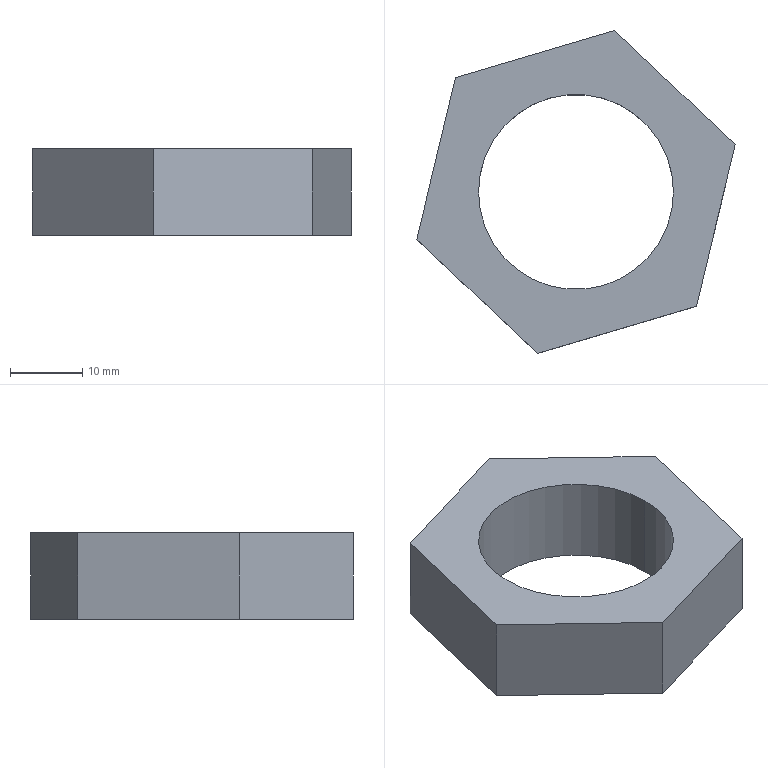Part | SolidWorks | features BaseBody 1 | 1 solid | 10 faces | box 44.103 x 44.731 x 12 mm | volume 9622 mm3 | plane 8 | cylinder 2 | commonest cylinder face diameters 27 x2
STEP:
#1=CARTESIAN_POINT('',(-24.66,14.233,12.));
#2=VERTEX_POINT('',#1);
#3=CARTESIAN_POINT('',(-51.66,14.233,12.));
#4=VERTEX_POINT('',#3);
#5=CARTESIAN_POINT('',(-38.16,14.233,12.));
#6=DIRECTION('',(0.,0.,-1.));
#7=DIRECTION('',(-1.,0.,0.));
#8=AXIS2_PLACEMENT_3D('',#5,#6,#7);
#9=CIRCLE('',#8,13.5);
#10=EDGE_CURVE('',#2,#4,#9,.T.);
#11=ORIENTED_EDGE('',*,*,#10,.F.);
#12=CARTESIAN_POINT('',(-24.66,14.233,0.));
#13=VERTEX_POINT('',#12);
#14=CARTESIAN_POINT('',(-24.66,14.233,12.));
#15=DIRECTION('',(0.,0.,-1.));
#16=VECTOR('',#15,1000.);
#17=LINE('',#14,#16);
#18=EDGE_CURVE('',#2,#13,#17,.T.);
#19=ORIENTED_EDGE('',*,*,#18,.T.);
#20=CARTESIAN_POINT('',(-51.66,14.233,0.));
#21=VERTEX_POINT('',#20);
#22=CARTESIAN_POINT('',(-38.16,14.233,0.));
#23=DIRECTION('',(0.,0.,1.));
#24=DIRECTION('',(-1.,0.,0.));
#25=AXIS2_PLACEMENT_3D('',#22,#23,#24);
#26=CIRCLE('',#25,13.5);
#27=EDGE_CURVE('',#21,#13,#26,.T.);
#28=ORIENTED_EDGE('',*,*,#27,.F.);
#29=CARTESIAN_POINT('',(-51.66,14.233,12.));
#30=DIRECTION('',(0.,0.,-1.));
#31=VECTOR('',#30,1000.);
#32=LINE('',#29,#31);
#33=EDGE_CURVE('',#4,#21,#32,.T.);
#34=ORIENTED_EDGE('',*,*,#33,.F.);
#35=EDGE_LOOP('',(#11,#19,#28,#34));
#36=FACE_OUTER_BOUND('',#35,.T.);
#37=CARTESIAN_POINT('',(-38.16,14.233,12.));
#38=DIRECTION('',(0.,0.,-1.));
#39=DIRECTION('',(-1.,0.,0.));
#40=AXIS2_PLACEMENT_3D('',#37,#38,#39);
#41=CYLINDRICAL_SURFACE('',#40,13.5);
#42=ADVANCED_FACE('',(#36),#41,.F.);
#43=CARTESIAN_POINT('',(-38.16,14.233,12.));
#44=DIRECTION('',(0.,0.,-1.));
#45=DIRECTION('',(-1.,0.,0.));
#46=AXIS2_PLACEMENT_3D('',#43,#44,#45);
#47=CIRCLE('',#46,13.5);
#48=EDGE_CURVE('',#4,#2,#47,.T.);
#49=ORIENTED_EDGE('',*,*,#48,.T.);
#50=ORIENTED_EDGE('',*,*,#10,.T.);
#51=EDGE_LOOP('',(#49,#50));
#52=FACE_BOUND('',#51,.T.);
#53=CARTESIAN_POINT('',(-54.847,30.062,12.));
#54=VERTEX_POINT('',#53);
#55=CARTESIAN_POINT('',(-60.211,7.696,12.));
#56=VERTEX_POINT('',#55);
#57=CARTESIAN_POINT('',(-54.847,30.062,12.));
#58=DIRECTION('',(-0.2332,-0.9724,0.));
#59=VECTOR('',#58,1000.);
#60=LINE('',#57,#59);
#61=EDGE_CURVE('',#54,#56,#60,.T.);
#62=ORIENTED_EDGE('',*,*,#61,.T.);
#63=CARTESIAN_POINT('',(-43.524,-8.133,12.));
#64=VERTEX_POINT('',#63);
#65=CARTESIAN_POINT('',(-60.211,7.696,12.));
#66=DIRECTION('',(0.7255,-0.6882,0.));
#67=VECTOR('',#66,1000.);
#68=LINE('',#65,#67);
#69=EDGE_CURVE('',#56,#64,#68,.T.);
#70=ORIENTED_EDGE('',*,*,#69,.T.);
#71=CARTESIAN_POINT('',(-21.473,-1.595,12.));
#72=VERTEX_POINT('',#71);
#73=CARTESIAN_POINT('',(-43.524,-8.133,12.));
#74=DIRECTION('',(0.9588,0.2842,0.));
#75=VECTOR('',#74,1000.);
#76=LINE('',#73,#75);
#77=EDGE_CURVE('',#64,#72,#76,.T.);
#78=ORIENTED_EDGE('',*,*,#77,.T.);
#79=CARTESIAN_POINT('',(-16.108,20.771,12.));
#80=VERTEX_POINT('',#79);
#81=CARTESIAN_POINT('',(-21.473,-1.595,12.));
#82=DIRECTION('',(0.2332,0.9724,0.));
#83=VECTOR('',#82,1000.);
#84=LINE('',#81,#83);
#85=EDGE_CURVE('',#72,#80,#84,.T.);
#86=ORIENTED_EDGE('',*,*,#85,.T.);
#87=CARTESIAN_POINT('',(-32.796,36.599,12.));
#88=VERTEX_POINT('',#87);
#89=CARTESIAN_POINT('',(-16.108,20.771,12.));
#90=DIRECTION('',(-0.7255,0.6882,0.));
#91=VECTOR('',#90,1000.);
#92=LINE('',#89,#91);
#93=EDGE_CURVE('',#80,#88,#92,.T.);
#94=ORIENTED_EDGE('',*,*,#93,.T.);
#95=CARTESIAN_POINT('',(-32.796,36.599,12.));
#96=DIRECTION('',(-0.9588,-0.2842,0.));
#97=VECTOR('',#96,1000.);
#98=LINE('',#95,#97);
#99=EDGE_CURVE('',#88,#54,#98,.T.);
#100=ORIENTED_EDGE('',*,*,#99,.T.);
#101=EDGE_LOOP('',(#62,#70,#78,#86,#94,#100));
#102=FACE_OUTER_BOUND('',#101,.T.);
#103=CARTESIAN_POINT('',(0.,0.,12.));
#104=DIRECTION('',(0.,0.,1.));
#105=DIRECTION('',(1.,0.,0.));
#106=AXIS2_PLACEMENT_3D('',#103,#104,#105);
#107=PLANE('',#106);
#108=ADVANCED_FACE('',(#52,#102),#107,.T.);
#109=ORIENTED_EDGE('',*,*,#18,.F.);
#110=ORIENTED_EDGE('',*,*,#48,.F.);
#111=ORIENTED_EDGE('',*,*,#33,.T.);
#112=CARTESIAN_POINT('',(-38.16,14.233,0.));
#113=DIRECTION('',(0.,0.,1.));
#114=DIRECTION('',(-1.,0.,0.));
#115=AXIS2_PLACEMENT_3D('',#112,#113,#114);
#116=CIRCLE('',#115,13.5);
#117=EDGE_CURVE('',#13,#21,#116,.T.);
#118=ORIENTED_EDGE('',*,*,#117,.F.);
#119=EDGE_LOOP('',(#109,#110,#111,#118));
#120=FACE_OUTER_BOUND('',#119,.T.);
#121=CARTESIAN_POINT('',(-38.16,14.233,12.));
#122=DIRECTION('',(0.,0.,-1.));
#123=DIRECTION('',(-1.,0.,0.));
#124=AXIS2_PLACEMENT_3D('',#121,#122,#123);
#125=CYLINDRICAL_SURFACE('',#124,13.5);
#126=ADVANCED_FACE('',(#120),#125,.F.);
#127=CARTESIAN_POINT('',(-43.524,-8.133,0.));
#128=VERTEX_POINT('',#127);
#129=CARTESIAN_POINT('',(-43.524,-8.133,12.));
#130=DIRECTION('',(0.,0.,-1.));
#131=VECTOR('',#130,1000.);
#132=LINE('',#129,#131);
#133=EDGE_CURVE('',#64,#128,#132,.T.);
#134=ORIENTED_EDGE('',*,*,#133,.F.);
#135=ORIENTED_EDGE('',*,*,#69,.F.);
#136=CARTESIAN_POINT('',(-60.211,7.696,0.));
#137=VERTEX_POINT('',#136);
#138=CARTESIAN_POINT('',(-60.211,7.696,12.));
#139=DIRECTION('',(0.,0.,1.));
#140=VECTOR('',#139,1000.);
#141=LINE('',#138,#140);
#142=EDGE_CURVE('',#137,#56,#141,.T.);
#143=ORIENTED_EDGE('',*,*,#142,.F.);
#144=CARTESIAN_POINT('',(-60.211,7.696,0.));
#145=DIRECTION('',(-0.7255,0.6882,0.));
#146=VECTOR('',#145,1000.);
#147=LINE('',#144,#146);
#148=EDGE_CURVE('',#128,#137,#147,.T.);
#149=ORIENTED_EDGE('',*,*,#148,.F.);
#150=EDGE_LOOP('',(#134,#135,#143,#149));
#151=FACE_OUTER_BOUND('',#150,.T.);
#152=CARTESIAN_POINT('',(-60.211,7.696,12.));
#153=DIRECTION('',(0.6882,0.7255,0.));
#154=DIRECTION('',(-0.7255,0.6882,0.));
#155=AXIS2_PLACEMENT_3D('',#152,#153,#154);
#156=PLANE('',#155);
#157=ADVANCED_FACE('',(#151),#156,.F.);
#158=ORIENTED_EDGE('',*,*,#142,.T.);
#159=ORIENTED_EDGE('',*,*,#61,.F.);
#160=CARTESIAN_POINT('',(-54.847,30.062,0.));
#161=VERTEX_POINT('',#160);
#162=CARTESIAN_POINT('',(-54.847,30.062,12.));
#163=DIRECTION('',(0.,0.,1.));
#164=VECTOR('',#163,1000.);
#165=LINE('',#162,#164);
#166=EDGE_CURVE('',#161,#54,#165,.T.);
#167=ORIENTED_EDGE('',*,*,#166,.F.);
#168=CARTESIAN_POINT('',(-54.847,30.062,0.));
#169=DIRECTION('',(0.2332,0.9724,0.));
#170=VECTOR('',#169,1000.);
#171=LINE('',#168,#170);
#172=EDGE_CURVE('',#137,#161,#171,.T.);
#173=ORIENTED_EDGE('',*,*,#172,.F.);
#174=EDGE_LOOP('',(#158,#159,#167,#173));
#175=FACE_OUTER_BOUND('',#174,.T.);
#176=CARTESIAN_POINT('',(-54.847,30.062,12.));
#177=DIRECTION('',(0.9724,-0.2332,0.));
#178=DIRECTION('',(0.2332,0.9724,0.));
#179=AXIS2_PLACEMENT_3D('',#176,#177,#178);
#180=PLANE('',#179);
#181=ADVANCED_FACE('',(#175),#180,.F.);
#182=ORIENTED_EDGE('',*,*,#166,.T.);
#183=ORIENTED_EDGE('',*,*,#99,.F.);
#184=CARTESIAN_POINT('',(-32.796,36.599,0.));
#185=VERTEX_POINT('',#184);
#186=CARTESIAN_POINT('',(-32.796,36.599,12.));
#187=DIRECTION('',(0.,0.,1.));
#188=VECTOR('',#187,1000.);
#189=LINE('',#186,#188);
#190=EDGE_CURVE('',#185,#88,#189,.T.);
#191=ORIENTED_EDGE('',*,*,#190,.F.);
#192=CARTESIAN_POINT('',(-32.796,36.599,0.));
#193=DIRECTION('',(0.9588,0.2842,0.));
#194=VECTOR('',#193,1000.);
#195=LINE('',#192,#194);
#196=EDGE_CURVE('',#161,#185,#195,.T.);
#197=ORIENTED_EDGE('',*,*,#196,.F.);
#198=EDGE_LOOP('',(#182,#183,#191,#197));
#199=FACE_OUTER_BOUND('',#198,.T.);
#200=CARTESIAN_POINT('',(-32.796,36.599,12.));
#201=DIRECTION('',(0.2842,-0.9588,0.));
#202=DIRECTION('',(0.9588,0.2842,0.));
#203=AXIS2_PLACEMENT_3D('',#200,#201,#202);
#204=PLANE('',#203);
#205=ADVANCED_FACE('',(#199),#204,.F.);
#206=ORIENTED_EDGE('',*,*,#190,.T.);
#207=ORIENTED_EDGE('',*,*,#93,.F.);
#208=CARTESIAN_POINT('',(-16.108,20.771,0.));
#209=VERTEX_POINT('',#208);
#210=CARTESIAN_POINT('',(-16.108,20.771,12.));
#211=DIRECTION('',(0.,0.,1.));
#212=VECTOR('',#211,1000.);
#213=LINE('',#210,#212);
#214=EDGE_CURVE('',#209,#80,#213,.T.);
#215=ORIENTED_EDGE('',*,*,#214,.F.);
#216=CARTESIAN_POINT('',(-16.108,20.771,0.));
#217=DIRECTION('',(0.7255,-0.6882,0.));
#218=VECTOR('',#217,1000.);
#219=LINE('',#216,#218);
#220=EDGE_CURVE('',#185,#209,#219,.T.);
#221=ORIENTED_EDGE('',*,*,#220,.F.);
#222=EDGE_LOOP('',(#206,#207,#215,#221));
#223=FACE_OUTER_BOUND('',#222,.T.);
#224=CARTESIAN_POINT('',(-16.108,20.771,12.));
#225=DIRECTION('',(-0.6882,-0.7255,0.));
#226=DIRECTION('',(0.7255,-0.6882,0.));
#227=AXIS2_PLACEMENT_3D('',#224,#225,#226);
#228=PLANE('',#227);
#229=ADVANCED_FACE('',(#223),#228,.F.);
#230=ORIENTED_EDGE('',*,*,#214,.T.);
#231=ORIENTED_EDGE('',*,*,#85,.F.);
#232=CARTESIAN_POINT('',(-21.473,-1.595,0.));
#233=VERTEX_POINT('',#232);
#234=CARTESIAN_POINT('',(-21.473,-1.595,12.));
#235=DIRECTION('',(0.,0.,1.));
#236=VECTOR('',#235,1000.);
#237=LINE('',#234,#236);
#238=EDGE_CURVE('',#233,#72,#237,.T.);
#239=ORIENTED_EDGE('',*,*,#238,.F.);
#240=CARTESIAN_POINT('',(-21.473,-1.595,0.));
#241=DIRECTION('',(-0.2332,-0.9724,0.));
#242=VECTOR('',#241,1000.);
#243=LINE('',#240,#242);
#244=EDGE_CURVE('',#209,#233,#243,.T.);
#245=ORIENTED_EDGE('',*,*,#244,.F.);
#246=EDGE_LOOP('',(#230,#231,#239,#245));
#247=FACE_OUTER_BOUND('',#246,.T.);
#248=CARTESIAN_POINT('',(-21.473,-1.595,12.));
#249=DIRECTION('',(-0.9724,0.2332,0.));
#250=DIRECTION('',(-0.2332,-0.9724,0.));
#251=AXIS2_PLACEMENT_3D('',#248,#249,#250);
#252=PLANE('',#251);
#253=ADVANCED_FACE('',(#247),#252,.F.);
#254=ORIENTED_EDGE('',*,*,#238,.T.);
#255=ORIENTED_EDGE('',*,*,#77,.F.);
#256=ORIENTED_EDGE('',*,*,#133,.T.);
#257=CARTESIAN_POINT('',(-43.524,-8.133,0.));
#258=DIRECTION('',(-0.9588,-0.2842,0.));
#259=VECTOR('',#258,1000.);
#260=LINE('',#257,#259);
#261=EDGE_CURVE('',#233,#128,#260,.T.);
#262=ORIENTED_EDGE('',*,*,#261,.F.);
#263=EDGE_LOOP('',(#254,#255,#256,#262));
#264=FACE_OUTER_BOUND('',#263,.T.);
#265=CARTESIAN_POINT('',(-43.524,-8.133,12.));
#266=DIRECTION('',(-0.2842,0.9588,0.));
#267=DIRECTION('',(-0.9588,-0.2842,0.));
#268=AXIS2_PLACEMENT_3D('',#265,#266,#267);
#269=PLANE('',#268);
#270=ADVANCED_FACE('',(#264),#269,.F.);
#271=ORIENTED_EDGE('',*,*,#27,.T.);
#272=ORIENTED_EDGE('',*,*,#117,.T.);
#273=EDGE_LOOP('',(#271,#272));
#274=FACE_BOUND('',#273,.T.);
#275=ORIENTED_EDGE('',*,*,#148,.T.);
#276=ORIENTED_EDGE('',*,*,#172,.T.);
#277=ORIENTED_EDGE('',*,*,#196,.T.);
#278=ORIENTED_EDGE('',*,*,#220,.T.);
#279=ORIENTED_EDGE('',*,*,#244,.T.);
#280=ORIENTED_EDGE('',*,*,#261,.T.);
#281=EDGE_LOOP('',(#275,#276,#277,#278,#279,#280));
#282=FACE_OUTER_BOUND('',#281,.T.);
#283=CARTESIAN_POINT('',(0.,0.,0.));
#284=DIRECTION('',(0.,0.,1.));
#285=DIRECTION('',(1.,0.,0.));
#286=AXIS2_PLACEMENT_3D('',#283,#284,#285);
#287=PLANE('',#286);
#288=ADVANCED_FACE('',(#274,#282),#287,.F.);
#289=CLOSED_SHELL('',(#42,#108,#126,#157,#181,#205,#229,#253,#270,#288));
#290=MANIFOLD_SOLID_BREP('',#289);
#291=CARTESIAN_POINT('',(0.,0.,0.));
#292=DIRECTION('',(0.,0.,1.));
#293=DIRECTION('',(1.,0.,0.));
#294=AXIS2_PLACEMENT_3D('',#291,#292,#293);
#295=(LENGTH_UNIT()NAMED_UNIT(*)SI_UNIT(.MILLI.,.METRE.));
#296=UNCERTAINTY_MEASURE_WITH_UNIT(LENGTH_MEASURE(0.00001),#295,'','');
#297=(NAMED_UNIT(*)PLANE_ANGLE_UNIT()SI_UNIT($,.RADIAN.));
#298=(NAMED_UNIT(*)SI_UNIT($,.STERADIAN.)SOLID_ANGLE_UNIT());
#299=(GEOMETRIC_REPRESENTATION_CONTEXT(3)GLOBAL_UNCERTAINTY_ASSIGNED_CONTEXT((#296))GLOBAL_UNIT_ASSIGNED_CONTEXT((#295,#297,#298))REPRESENTATION_CONTEXT('',''));
#300=ADVANCED_BREP_SHAPE_REPRESENTATION('',(#290,#294),#299);